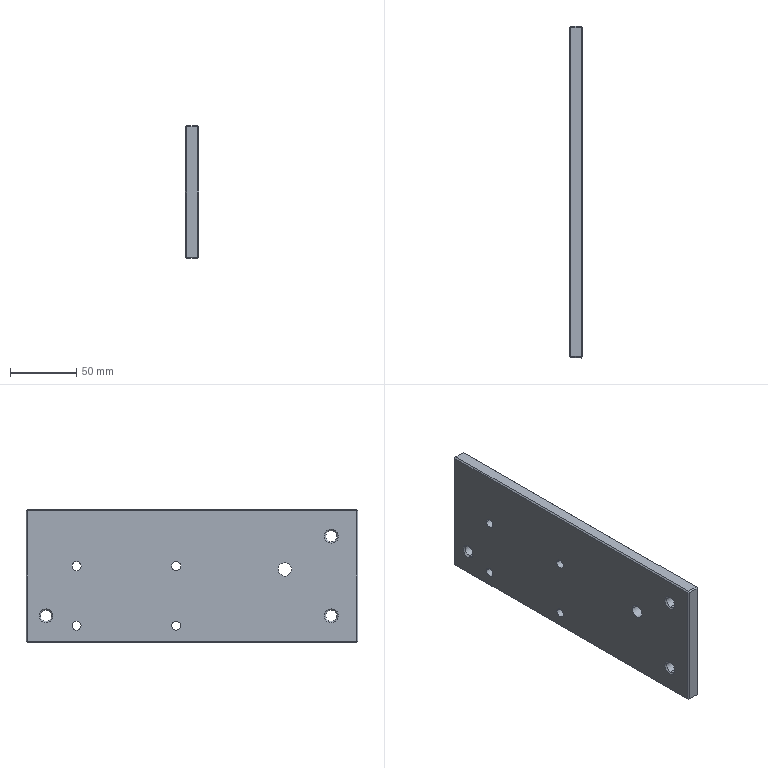Part | STEP file | 01-14 Caster foot cup support plate | 1 solid | 54 faces | box 10 x 250 x 100 mm | volume 245227 mm3 | plane 26 | cylinder 16 | cone 12 | commonest cylinder face diameters 6.8 x8 8.5 x6 10.2 x2